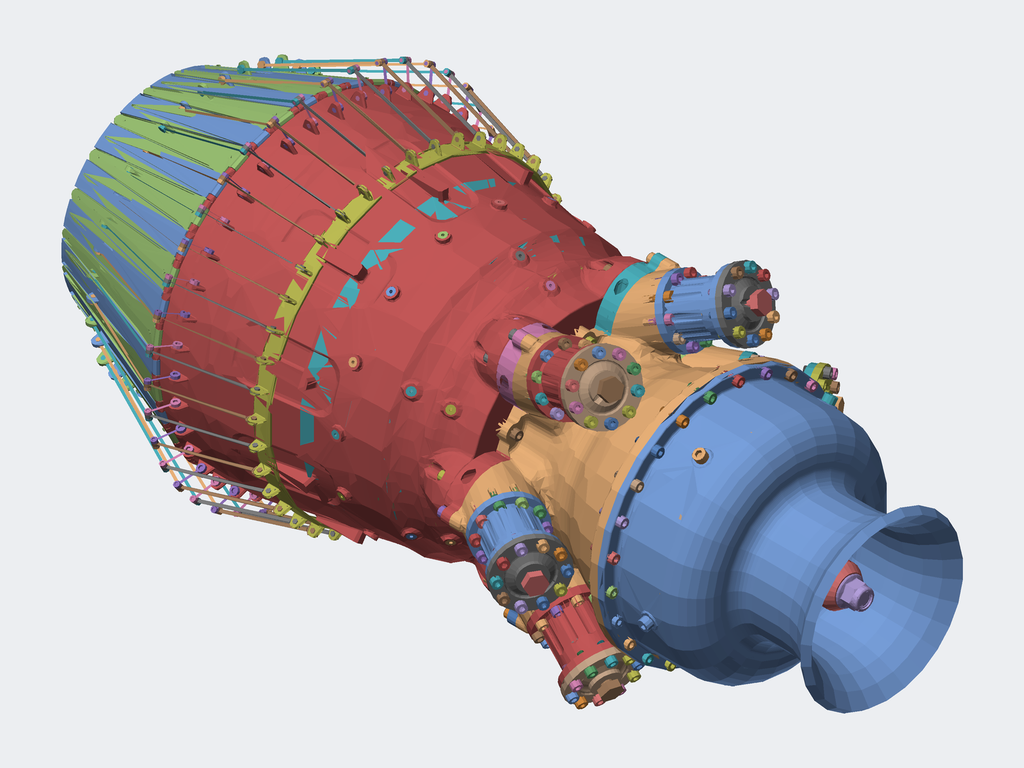Assembly | STEP file | 365 different items | 517 placed
Parts list (item | name | quantity | parent item | size | volume), first 214 of 365 items:
1 | Completa.sldasm-Part-1_Valor predeterminado (subassembly) | x1 | in Completa | 29.178 x 23 x 23 mm | 4698 mm3
2 | Completa.sldasm-Part-2_Valor predeterminado (subassembly) | x1 | in Completa | 40.919 x 104.793 x 101.882 mm | 59946 mm3
3 | Completa.sldasm-Part-3_Valor predeterminado (subassembly) | x1 | in Completa | 94.392 x 66 x 66 mm | 40484 mm3
4 | Completa.sldasm-Part-4_Valor predeterminado (subassembly) | x1 | in Completa | 21.228 x 16 x 16 mm | 1867 mm3
5 | Completa.sldasm-Part-5_Valor predeterminado (subassembly) | x1 | in Completa | 64.439 x 12 x 12 mm | 6023 mm3
6 | Completa.sldasm-Part-6_Valor predeterminado (subassembly) | x1 | in Completa | 23.351 x 16 x 16 mm | 2054 mm3
7 | Completa.sldasm-Part-7_Valor predeterminado (subassembly) | x1 | in Completa | 21.228 x 16 x 16 mm | 1867 mm3
8 | Completa.sldasm-Part-8_Valor predeterminado (subassembly) | x1 | in Completa | 64.439 x 12 x 12 mm | 6023 mm3
9 | Completa.sldasm-Part-9_Valor predeterminado (subassembly) | x1 | in Completa | 23.351 x 16 x 16 mm | 2054 mm3
10 | Completa.sldasm-Part-10_Valor predeterminado (subassembly) | x1 | in Completa | 21.228 x 16 x 16 mm | 1867 mm3
11 | Completa.sldasm-Part-11_Valor predeterminado (subassembly) | x1 | in Completa | 64.439 x 12 x 12 mm | 6023 mm3
12 | Completa.sldasm-Part-12_Valor predeterminado (subassembly) | x1 | in Completa | 23.351 x 16 x 16 mm | 2054 mm3
13 | Completa.sldasm-Part-13_Valor predeterminado (subassembly) | x1 | in Completa | 21.228 x 16 x 16 mm | 1867 mm3
14 | Completa.sldasm-Part-14_Valor predeterminado (subassembly) | x1 | in Completa | 64.439 x 12 x 12 mm | 6023 mm3
15 | Completa.sldasm-Part-15_Valor predeterminado (subassembly) | x1 | in Completa | 23.351 x 16 x 16 mm | 2054 mm3
16 | Completa.sldasm-Part-16_Valor predeterminado (subassembly) | x1 | in Completa | 23.351 x 16 x 16 mm | 2054 mm3
17 | Completa.sldasm-Part-17_Valor predeterminado (subassembly) | x1 | in Completa | 21.228 x 16 x 16 mm | 1867 mm3
18 | Completa.sldasm-Part-18_Valor predeterminado (subassembly) | x1 | in Completa | 64.439 x 12 x 12 mm | 6023 mm3
19 | Completa.sldasm-Part-19_Valor predeterminado (subassembly) | x1 | in Completa | 15.548 x 234.027 x 234.027 mm | 234749 mm3
20 | Completa.sldasm-Part-20_Valor predeterminado (subassembly) | x1 | in Completa | 7.542 x 74.256 x 74.256 mm | 20001 mm3
21 | Completa.sldasm-Part-21_Valor predeterminado (subassembly) | x1 | in Completa | 10 x 104.793 x 101.882 mm | 47802 mm3
22 | Completa.sldasm-Part-22_Valor predeterminado (subassembly) | x1 | in Completa | 260.435 x 179.116 x 179.116 mm | 192197 mm3
23 | Socket Countersunk Head Screw_ISO(ISO 10642 - M6 x 25 --- 25S)_Valor predeterminado | x1 | in Completa | 11.34 x 25.708 x 19.731 mm | 759.97 mm3
24 | Socket Countersunk Head Screw_ISO(ISO 10642 - M6 x 25 --- 25S)-1_Valor predeterminado | x1 | in Completa | 11.34 x 25.708 x 19.731 mm | 759.97 mm3
25 | Socket Countersunk Head Screw_ISO(ISO 10642 - M6 x 25 --- 25S)-2_Valor predeterminado | x1 | in Completa | 11.34 x 11.34 x 25 mm | 759.97 mm3
26 | Completa.sldasm-Part-23_Valor predeterminado (subassembly) | x1 | in Completa | 54.453 x 255.658 x 255.658 mm | 510804 mm3
27 | Completa.sldasm-Part-24_Valor predeterminado (subassembly) | x1 | in Completa | 132.616 x 276.232 x 245.091 mm | 834308 mm3
28 | Completa.sldasm-Part-25_Valor predeterminado (subassembly) | x1 | in Completa | 164.604 x 227.494 x 227.494 mm | 716979 mm3
29 | Completa.sldasm-Part-26_Valor predeterminado (subassembly) | x1 | in Completa | 13.228 x 193 x 193 mm | 129234 mm3
30 | Completa.sldasm-Part-27_Valor predeterminado (subassembly) | x1 | in Completa | 14 x 212.474 x 212.474 mm | 171916 mm3
31 | Torque nut 04-2_ISO(ISO 7043-M12-N)_Valor predeterminado | x1 | in Completa | 16.1 x 26 x 26 mm | 3173 mm3
32 | Socket Head Cap Screw_ISO(ISO 4762 M6 x 25 --- 25S)_Valor predeterminado | x1 | in Completa | 10 x 31.522 x 18.292 mm | 1014 mm3
33 | Socket Countersunk Head Screw_ISO(ISO 10642 - M6 x 25 --- 25S)-3_Valor predeterminado | x1 | in Completa | 25 x 11.34 x 11.34 mm | 759.97 mm3
34 | Socket Head Cap Screw_ISO(ISO 4762 M5 x 20 --- 20S)_Valor predeterminado | x1 | in Completa | 25 x 8.5 x 8.5 mm | 588.412 mm3
35 | Socket Head Cap Screw_ISO(ISO 4762 M5 x 20 --- 20S)-1_Valor predeterminado | x1 | in Completa | 25 x 8.5 x 8.5 mm | 588.412 mm3
36 | Socket Head Cap Screw_ISO(ISO 4762 M5 x 20 --- 20S)-2_Valor predeterminado | x1 | in Completa | 25 x 8.5 x 8.5 mm | 588.412 mm3
37 | Socket Head Cap Screw_ISO(ISO 4762 M5 x 20 --- 20S)-3_Valor predeterminado | x1 | in Completa | 25 x 8.5 x 8.5 mm | 588.412 mm3
38 | Socket Head Cap Screw_ISO(ISO 4762 M5 x 20 --- 20S)-4_Valor predeterminado | x1 | in Completa | 25 x 8.5 x 8.5 mm | 588.412 mm3
39 | Socket Head Cap Screw_ISO(ISO 4762 M5 x 20 --- 20S)-5_Valor predeterminado | x1 | in Completa | 25 x 8.5 x 8.5 mm | 588.412 mm3
40 | Socket Head Cap Screw_ISO(ISO 4762 M5 x 20 --- 20S)-6_Valor predeterminado | x1 | in Completa | 25 x 8.5 x 8.5 mm | 588.412 mm3
41 | Socket Head Cap Screw_ISO(ISO 4762 M5 x 20 --- 20S)-7_Valor predeterminado | x1 | in Completa | 25 x 8.5 x 8.5 mm | 588.412 mm3
42 | Previa 01.sldasm-Part-10_Valor predeterminado (subassembly) | x1 | in Completa | 66 x 12 x 12 mm | 6169 mm3
43 | Previa 01.sldasm-Part-16_Valor predeterminado (subassembly) | x1 | in Completa | 21.5 x 177.565 x 177.455 mm | 157095 mm3
44 | Previa 01.sldasm-Part-15_Valor predeterminado (subassembly) | x1 | in Completa | 24.229 x 188.642 x 188.976 mm | 257389 mm3
45 | Previa 01.sldasm-Part-14_Valor predeterminado (subassembly) | x1 | in Completa | 19 x 165.343 x 165.042 mm | 149848 mm3
46 | Previa 01.sldasm-Part-13_Valor predeterminado (subassembly) | x1 | in Completa | 8 x 36.3 x 36.3 mm | 5808 mm3
47 | Previa 01.sldasm-Part-11_Valor predeterminado (subassembly) | x1 | in Completa | 7 x 37.038 x 37.038 mm | 5630 mm3
48 | 003.sldasm-Part-1_Valor predeterminado (subassembly) | x1 | in Completa | 26.301 x 191 x 190.919 mm | 221330 mm3
49 | Previa 01.sldasm-Part-5_Valor predeterminado (subassembly) | x1 | in Completa | 26 x 108 x 108 mm | 90690 mm3
50 | Previa 01.sldasm-Part-4_Valor predeterminado (subassembly) | x1 | in Completa | 26.228 x 190 x 189.8 mm | 157872 mm3
51 | 003.sldasm-Part-2_Valor predeterminado (subassembly) | x1 | in Completa | 11 x 91.038 x 91.038 mm | 45789 mm3
52 | Previa 01.sldasm-Part-1_Valor predeterminado (subassembly) | x1 | in Completa | - | 182355 mm3
53 | Socket Head Cap Screw_ISO(ISO 4762 M5 x 20 --- 20S)-8_Valor predeterminado | x1 | in Completa | 19.995 x 15.067 x 8.5 mm | 493.761 mm3
54 | Socket Head Cap Screw_ISO(ISO 4762 M5 x 20 --- 20S)-9_Valor predeterminado | x1 | in Completa | 19.995 x 15.067 x 8.5 mm | 493.761 mm3
55 | Socket Head Cap Screw_ISO(ISO 4762 M5 x 20 --- 20S)-10_Valor predeterminado | x1 | in Completa | 19.995 x 15.067 x 8.5 mm | 493.761 mm3
56 | Socket Head Cap Screw_ISO(ISO 4762 M5 x 20 --- 20S)-11_Valor predeterminado | x1 | in Completa | 19.995 x 15.067 x 8.5 mm | 493.761 mm3
57 | Socket Head Cap Screw_ISO(ISO 4762 M5 x 20 --- 20S)-12_Valor predeterminado | x1 | in Completa | 19.995 x 15.067 x 8.5 mm | 493.761 mm3
58 | Socket Head Cap Screw_ISO(ISO 4762 M5 x 20 --- 20S)-13_Valor predeterminado | x1 | in Completa | 19.995 x 15.067 x 8.5 mm | 493.761 mm3
59 | Socket Head Cap Screw_ISO(ISO 4762 M5 x 20 --- 20S)-14_Valor predeterminado | x1 | in Completa | 19.995 x 15.067 x 8.5 mm | 493.761 mm3
60 | Socket Head Cap Screw_ISO(ISO 4762 M5 x 20 --- 20S)-15_Valor predeterminado | x1 | in Completa | 19.995 x 15.067 x 8.5 mm | 493.761 mm3
61 | Socket Head Cap Screw_ISO(ISO 4762 M5 x 20 --- 20S)-16_Valor predeterminado | x1 | in Completa | 19.995 x 15.067 x 8.5 mm | 493.761 mm3
62 | Socket Head Cap Screw_ISO(ISO 4762 M5 x 20 --- 20S)-17_Valor predeterminado | x1 | in Completa | 19.995 x 15.067 x 8.5 mm | 493.761 mm3
63 | Socket Head Cap Screw_ISO(ISO 4762 M5 x 20 --- 20S)-18_Valor predeterminado | x1 | in Completa | 24.833 x 17.717 x 8.5 mm | 588.412 mm3
64 | Socket Head Cap Screw_ISO(ISO 4762 M5 x 20 --- 20S)-19_Valor predeterminado | x1 | in Completa | 24.833 x 17.717 x 8.5 mm | 588.412 mm3
65 | Socket Head Cap Screw_ISO(ISO 4762 M5 x 20 --- 20S)-20_Valor predeterminado | x1 | in Completa | 24.833 x 17.717 x 8.5 mm | 588.412 mm3
66 | Socket Head Cap Screw_ISO(ISO 4762 M5 x 20 --- 20S)-21_Valor predeterminado | x1 | in Completa | 24.833 x 17.717 x 8.5 mm | 588.412 mm3
67 | Socket Head Cap Screw_ISO(ISO 4762 M5 x 20 --- 20S)-22_Valor predeterminado | x1 | in Completa | 24.833 x 17.717 x 8.5 mm | 588.412 mm3
68 | Socket Head Cap Screw_ISO(ISO 4762 M5 x 20 --- 20S)-23_Valor predeterminado | x1 | in Completa | 24.833 x 17.717 x 8.5 mm | 588.412 mm3
69 | Socket Head Cap Screw_ISO(ISO 4762 M5 x 20 --- 20S)-24_Valor predeterminado | x1 | in Completa | 24.833 x 17.717 x 8.5 mm | 588.412 mm3
70 | Socket Head Cap Screw_ISO(ISO 4762 M5 x 20 --- 20S)-25_Valor predeterminado | x1 | in Completa | 24.833 x 17.717 x 8.5 mm | 588.412 mm3
71 | Socket Head Cap Screw_ISO(ISO 4762 M5 x 20 --- 20S)-26_Valor predeterminado | x1 | in Completa | 24.833 x 17.717 x 8.5 mm | 588.412 mm3
72 | Socket Head Cap Screw_ISO(ISO 4762 M5 x 20 --- 20S)-27_Valor predeterminado | x1 | in Completa | 24.833 x 17.717 x 8.5 mm | 588.412 mm3
73 | Completa.sldasm-Part-28_Valor predeterminado (subassembly) | x1 | in Completa | 33.841 x 55.116 x 60 mm | 15153 mm3
74 | Completa.sldasm-Part-29_Valor predeterminado (subassembly) | x1 | in Completa | 74.277 x 76.616 x 59 mm | 34566 mm3
75 | Completa.sldasm-Part-30_Valor predeterminado (subassembly) | x1 | in Completa | 34.045 x 26.016 x 16 mm | 3225 mm3
76 | Completa.sldasm-Part-31_Valor predeterminado (subassembly) | x1 | in Completa | 97.324 x 73.886 x 36.376 mm | 6808 mm3
77 | Socket Countersunk Head Screw_ISO(ISO 10642 - M6 x 25 --- 25S)-4_Valor predeterminado | x1 | in Completa | 25 x 11.34 x 11.34 mm | 759.97 mm3
78 | Socket Countersunk Head Screw_ISO(ISO 10642 - M6 x 25 --- 25S)-5_Valor predeterminado | x1 | in Completa | 25 x 11.34 x 11.34 mm | 759.97 mm3
79 | Previa 01.sldasm-Part-10-1_Valor predeterminado (subassembly) | x1 | in Completa | 66 x 12 x 12 mm | 6169 mm3
80 | Socket Countersunk Head Screw_ISO(ISO 10642 - M6 x 25 --- 25S)-6_Valor predeterminado | x1 | in Completa | 25 x 11.34 x 11.34 mm | 759.97 mm3
81 | Socket Countersunk Head Screw_ISO(ISO 10642 - M6 x 25 --- 25S)-7_Valor predeterminado | x1 | in Completa | 25 x 11.34 x 11.34 mm | 759.97 mm3
82 | Previa 01.sldasm-Part-10-2_Valor predeterminado (subassembly) | x1 | in Completa | 66 x 12 x 12 mm | 6169 mm3
83 | Socket Countersunk Head Screw_ISO(ISO 10642 - M6 x 25 --- 25S)-8_Valor predeterminado | x1 | in Completa | 25 x 11.34 x 11.34 mm | 759.97 mm3
84 | Socket Countersunk Head Screw_ISO(ISO 10642 - M6 x 25 --- 25S)-9_Valor predeterminado | x1 | in Completa | 25 x 11.34 x 11.34 mm | 759.97 mm3
85 | Previa 01.sldasm-Part-10-3_Valor predeterminado (subassembly) | x1 | in Completa | 66 x 12 x 12 mm | 6169 mm3
86 | Socket Countersunk Head Screw_ISO(ISO 10642 - M6 x 25 --- 25S)-10_Valor predeterminado | x1 | in Completa | 25 x 11.34 x 11.34 mm | 759.97 mm3
87 | Socket Countersunk Head Screw_ISO(ISO 10642 - M6 x 25 --- 25S)-11_Valor predeterminado | x1 | in Completa | 25 x 11.34 x 11.34 mm | 759.97 mm3
88 | Previa 01.sldasm-Part-10-4_Valor predeterminado (subassembly) | x1 | in Completa | 66 x 12 x 12 mm | 6169 mm3
89 | Socket Countersunk Head Screw_ISO(ISO 10642 - M6 x 25 --- 25S)-12_Valor predeterminado | x1 | in Completa | 25 x 11.34 x 11.34 mm | 759.97 mm3
90 | Socket Head Cap Screw_ISO(ISO 4762 M6 x 25 --- 25S)-1_Valor predeterminado | x1 | in Completa | 10 x 25.255 x 28.655 mm | 1014 mm3
91 | Socket Head Cap Screw_ISO(ISO 4762 M6 x 25 --- 25S)-2_Valor predeterminado | x1 | in Completa | 10 x 23.176 x 29.939 mm | 1014 mm3
92 | Socket Head Cap Screw_ISO(ISO 4762 M6 x 25 --- 25S)-3_Valor predeterminado | x1 | in Completa | 10 x 31.803 x 15.54 mm | 1014 mm3
93 | Socket Head Cap Screw_ISO(ISO 4762 M6 x 25 --- 25S)-4_Valor predeterminado | x1 | in Completa | 10 x 10.285 x 31.332 mm | 1014 mm3
94 | Socket Head Cap Screw_ISO(ISO 4762 M5 x 20 --- 20S)-28_Valor predeterminado | x1 | in Completa | 24.833 x 12.447 x 16.353 mm | 588.412 mm3
95 | Socket Head Cap Screw_ISO(ISO 4762 M5 x 20 --- 20S)-29_Valor predeterminado | x1 | in Completa | 19.995 x 11.122 x 14.058 mm | 493.761 mm3
96 | Socket Head Cap Screw_ISO(ISO 4762 M5 x 20 --- 20S)-30_Valor predeterminado | x1 | in Completa | 24.833 x 12.447 x 16.353 mm | 588.412 mm3
97 | Socket Head Cap Screw_ISO(ISO 4762 M5 x 20 --- 20S)-31_Valor predeterminado | x1 | in Completa | 19.995 x 11.122 x 14.058 mm | 493.761 mm3
98 | Socket Head Cap Screw_ISO(ISO 4762 M5 x 20 --- 20S)-32_Valor predeterminado | x1 | in Completa | 19.995 x 11.122 x 14.058 mm | 493.761 mm3
99 | Socket Head Cap Screw_ISO(ISO 4762 M5 x 20 --- 20S)-33_Valor predeterminado | x1 | in Completa | 24.833 x 12.447 x 16.353 mm | 588.412 mm3
100 | Socket Head Cap Screw_ISO(ISO 4762 M5 x 20 --- 20S)-34_Valor predeterminado | x1 | in Completa | 19.995 x 11.122 x 14.058 mm | 493.761 mm3
101 | Socket Head Cap Screw_ISO(ISO 4762 M5 x 20 --- 20S)-35_Valor predeterminado | x1 | in Completa | 24.833 x 12.447 x 16.353 mm | 588.412 mm3
102 | Socket Head Cap Screw_ISO(ISO 4762 M5 x 20 --- 20S)-36_Valor predeterminado | x1 | in Completa | 19.995 x 11.122 x 14.058 mm | 493.761 mm3
103 | Socket Head Cap Screw_ISO(ISO 4762 M5 x 20 --- 20S)-37_Valor predeterminado | x1 | in Completa | 24.833 x 12.447 x 16.353 mm | 588.412 mm3
104 | Completa.sldasm-Part-32_Valor predeterminado (subassembly) | x1 | in Completa | 33.841 x 59.529 x 56.74 mm | 15153 mm3
105 | Socket Head Cap Screw_ISO(ISO 4762 M5 x 20 --- 20S)-38_Valor predeterminado | x1 | in Completa | 19.995 x 11.122 x 14.058 mm | 493.761 mm3
106 | Socket Head Cap Screw_ISO(ISO 4762 M5 x 20 --- 20S)-39_Valor predeterminado | x1 | in Completa | 19.995 x 11.122 x 14.058 mm | 493.761 mm3
107 | Socket Head Cap Screw_ISO(ISO 4762 M5 x 20 --- 20S)-40_Valor predeterminado | x1 | in Completa | 19.995 x 11.122 x 14.058 mm | 493.761 mm3
108 | Completa.sldasm-Part-33_Valor predeterminado (subassembly) | x1 | in Completa | 74.277 x 69.48 x 75.135 mm | 34566 mm3
109 | Socket Head Cap Screw_ISO(ISO 4762 M5 x 20 --- 20S)-41_Valor predeterminado | x1 | in Completa | 24.833 x 12.447 x 16.353 mm | 588.412 mm3
110 | Completa.sldasm-Part-34_Valor predeterminado (subassembly) | x1 | in Completa | 34.045 x 21.356 x 23.621 mm | 3225 mm3
111 | Socket Head Cap Screw_ISO(ISO 4762 M5 x 20 --- 20S)-42_Valor predeterminado | x1 | in Completa | 19.995 x 11.122 x 14.058 mm | 493.761 mm3
112 | Completa.sldasm-Part-35_Valor predeterminado (subassembly) | x1 | in Completa | 97.324 x 59.709 x 73.971 mm | 6808 mm3
113 | Socket Head Cap Screw_ISO(ISO 4762 M5 x 20 --- 20S)-43_Valor predeterminado | x1 | in Completa | 19.995 x 11.122 x 14.058 mm | 493.761 mm3
114 | Socket Head Cap Screw_ISO(ISO 4762 M5 x 20 --- 20S)-44_Valor predeterminado | x1 | in Completa | 24.833 x 12.447 x 16.353 mm | 588.412 mm3
115 | Socket Head Cap Screw_ISO(ISO 4762 M5 x 20 --- 20S)-45_Valor predeterminado | x1 | in Completa | 24.833 x 12.447 x 16.353 mm | 588.412 mm3
116 | Socket Head Cap Screw_ISO(ISO 4762 M5 x 20 --- 20S)-46_Valor predeterminado | x1 | in Completa | 24.833 x 12.447 x 16.353 mm | 588.412 mm3
117 | Socket Head Cap Screw_ISO(ISO 4762 M5 x 20 --- 20S)-47_Valor predeterminado | x1 | in Completa | 24.833 x 12.447 x 16.353 mm | 588.412 mm3
118 | Socket Head Cap Screw_ISO(ISO 4762 M5 x 20 --- 20S)-48_Valor predeterminado | x1 | in Completa | 24.833 x 12.447 x 16.353 mm | 588.412 mm3
119 | Socket Head Cap Screw_ISO(ISO 4762 M5 x 20 --- 20S)-49_Valor predeterminado | x1 | in Completa | 19.995 x 11.122 x 14.058 mm | 493.761 mm3
120 | Socket Head Cap Screw_ISO(ISO 4762 M5 x 20 --- 20S)-50_Valor predeterminado | x1 | in Completa | 24.833 x 12.447 x 16.353 mm | 588.412 mm3
121 | Socket Head Cap Screw_ISO(ISO 4762 M5 x 20 --- 20S)-51_Valor predeterminado | x1 | in Completa | 19.995 x 11.122 x 14.058 mm | 493.761 mm3
122 | Socket Head Cap Screw_ISO(ISO 4762 M5 x 20 --- 20S)-52_Valor predeterminado | x1 | in Completa | 19.995 x 11.122 x 14.058 mm | 493.761 mm3
123 | Socket Head Cap Screw_ISO(ISO 4762 M5 x 20 --- 20S)-53_Valor predeterminado | x1 | in Completa | 24.833 x 12.447 x 16.353 mm | 588.412 mm3
124 | Socket Head Cap Screw_ISO(ISO 4762 M5 x 20 --- 20S)-54_Valor predeterminado | x1 | in Completa | 19.995 x 11.122 x 14.058 mm | 493.761 mm3
125 | Socket Head Cap Screw_ISO(ISO 4762 M5 x 20 --- 20S)-55_Valor predeterminado | x1 | in Completa | 24.833 x 12.447 x 16.353 mm | 588.412 mm3
126 | Socket Head Cap Screw_ISO(ISO 4762 M5 x 20 --- 20S)-56_Valor predeterminado | x1 | in Completa | 19.995 x 11.122 x 14.058 mm | 493.761 mm3
127 | Socket Head Cap Screw_ISO(ISO 4762 M5 x 20 --- 20S)-57_Valor predeterminado | x1 | in Completa | 24.833 x 12.447 x 16.353 mm | 588.412 mm3
128 | Completa.sldasm-Part-36_Valor predeterminado (subassembly) | x1 | in Completa | 33.841 x 59.529 x 56.74 mm | 15153 mm3
129 | Socket Head Cap Screw_ISO(ISO 4762 M5 x 20 --- 20S)-58_Valor predeterminado | x1 | in Completa | 19.995 x 11.122 x 14.058 mm | 493.761 mm3
130 | Socket Head Cap Screw_ISO(ISO 4762 M5 x 20 --- 20S)-59_Valor predeterminado | x1 | in Completa | 19.995 x 11.122 x 14.058 mm | 493.761 mm3
131 | Socket Head Cap Screw_ISO(ISO 4762 M5 x 20 --- 20S)-60_Valor predeterminado | x1 | in Completa | 19.995 x 11.122 x 14.058 mm | 493.761 mm3
132 | Completa.sldasm-Part-37_Valor predeterminado (subassembly) | x1 | in Completa | 74.277 x 69.48 x 75.135 mm | 34566 mm3
133 | Socket Head Cap Screw_ISO(ISO 4762 M5 x 20 --- 20S)-61_Valor predeterminado | x1 | in Completa | 24.833 x 12.447 x 16.353 mm | 588.412 mm3
134 | Completa.sldasm-Part-38_Valor predeterminado (subassembly) | x1 | in Completa | 34.045 x 21.356 x 23.621 mm | 3225 mm3
135 | Socket Head Cap Screw_ISO(ISO 4762 M5 x 20 --- 20S)-62_Valor predeterminado | x1 | in Completa | 19.995 x 11.122 x 14.058 mm | 493.761 mm3
136 | Completa.sldasm-Part-39_Valor predeterminado (subassembly) | x1 | in Completa | 97.324 x 59.709 x 73.971 mm | 6808 mm3
137 | Socket Head Cap Screw_ISO(ISO 4762 M5 x 20 --- 20S)-63_Valor predeterminado | x1 | in Completa | 19.995 x 11.122 x 14.058 mm | 493.761 mm3
138 | Socket Head Cap Screw_ISO(ISO 4762 M5 x 20 --- 20S)-64_Valor predeterminado | x1 | in Completa | 24.833 x 12.447 x 16.353 mm | 588.412 mm3
139 | Socket Head Cap Screw_ISO(ISO 4762 M5 x 20 --- 20S)-65_Valor predeterminado | x1 | in Completa | 24.833 x 12.447 x 16.353 mm | 588.412 mm3
140 | Socket Head Cap Screw_ISO(ISO 4762 M5 x 20 --- 20S)-66_Valor predeterminado | x1 | in Completa | 24.833 x 12.447 x 16.353 mm | 588.412 mm3
141 | Socket Head Cap Screw_ISO(ISO 4762 M5 x 20 --- 20S)-67_Valor predeterminado | x1 | in Completa | 24.833 x 12.447 x 16.353 mm | 588.412 mm3
142 | Socket Head Cap Screw_ISO(ISO 4762 M5 x 20 --- 20S)-68_Valor predeterminado | x1 | in Completa | 24.833 x 17.717 x 8.5 mm | 588.412 mm3
143 | Socket Head Cap Screw_ISO(ISO 4762 M5 x 20 --- 20S)-69_Valor predeterminado | x1 | in Completa | 19.995 x 15.067 x 8.5 mm | 493.761 mm3
144 | Socket Head Cap Screw_ISO(ISO 4762 M5 x 20 --- 20S)-70_Valor predeterminado | x1 | in Completa | 24.833 x 17.717 x 8.5 mm | 588.412 mm3
145 | Socket Head Cap Screw_ISO(ISO 4762 M5 x 20 --- 20S)-71_Valor predeterminado | x1 | in Completa | 19.995 x 15.067 x 8.5 mm | 493.761 mm3
146 | Socket Head Cap Screw_ISO(ISO 4762 M5 x 20 --- 20S)-72_Valor predeterminado | x1 | in Completa | 19.995 x 15.067 x 8.5 mm | 493.761 mm3
147 | Socket Head Cap Screw_ISO(ISO 4762 M5 x 20 --- 20S)-73_Valor predeterminado | x1 | in Completa | 24.833 x 17.717 x 8.5 mm | 588.412 mm3
148 | Socket Head Cap Screw_ISO(ISO 4762 M5 x 20 --- 20S)-74_Valor predeterminado | x1 | in Completa | 19.995 x 15.067 x 8.5 mm | 493.761 mm3
149 | Socket Head Cap Screw_ISO(ISO 4762 M5 x 20 --- 20S)-75_Valor predeterminado | x1 | in Completa | 24.833 x 17.717 x 8.5 mm | 588.412 mm3
150 | Socket Head Cap Screw_ISO(ISO 4762 M5 x 20 --- 20S)-76_Valor predeterminado | x1 | in Completa | 19.995 x 15.067 x 8.5 mm | 493.761 mm3
151 | Socket Head Cap Screw_ISO(ISO 4762 M5 x 20 --- 20S)-77_Valor predeterminado | x1 | in Completa | 24.833 x 17.717 x 8.5 mm | 588.412 mm3
152 | Completa.sldasm-Part-40_Valor predeterminado (subassembly) | x1 | in Completa | 33.841 x 55.116 x 60 mm | 15153 mm3
153 | Socket Head Cap Screw_ISO(ISO 4762 M5 x 20 --- 20S)-78_Valor predeterminado | x1 | in Completa | 19.995 x 15.067 x 8.5 mm | 493.761 mm3
154 | Socket Head Cap Screw_ISO(ISO 4762 M5 x 20 --- 20S)-79_Valor predeterminado | x1 | in Completa | 19.995 x 15.067 x 8.5 mm | 493.761 mm3
155 | Socket Head Cap Screw_ISO(ISO 4762 M5 x 20 --- 20S)-80_Valor predeterminado | x1 | in Completa | 19.995 x 15.067 x 8.5 mm | 493.761 mm3
156 | Completa.sldasm-Part-41_Valor predeterminado (subassembly) | x1 | in Completa | 74.277 x 76.616 x 59 mm | 34566 mm3
157 | Socket Head Cap Screw_ISO(ISO 4762 M5 x 20 --- 20S)-81_Valor predeterminado | x1 | in Completa | 24.833 x 17.717 x 8.5 mm | 588.412 mm3
158 | Completa.sldasm-Part-42_Valor predeterminado (subassembly) | x1 | in Completa | 34.045 x 26.016 x 16 mm | 3225 mm3
159 | Socket Head Cap Screw_ISO(ISO 4762 M5 x 20 --- 20S)-82_Valor predeterminado | x1 | in Completa | 19.995 x 15.067 x 8.5 mm | 493.761 mm3
160 | Completa.sldasm-Part-43_Valor predeterminado (subassembly) | x1 | in Completa | 97.324 x 73.886 x 36.376 mm | 6808 mm3
161 | Socket Head Cap Screw_ISO(ISO 4762 M5 x 20 --- 20S)-83_Valor predeterminado | x1 | in Completa | 19.995 x 15.067 x 8.5 mm | 493.761 mm3
162 | Socket Head Cap Screw_ISO(ISO 4762 M5 x 20 --- 20S)-84_Valor predeterminado | x1 | in Completa | 24.833 x 17.717 x 8.5 mm | 588.412 mm3
163 | Socket Head Cap Screw_ISO(ISO 4762 M5 x 20 --- 20S)-85_Valor predeterminado | x1 | in Completa | 24.833 x 17.717 x 8.5 mm | 588.412 mm3
164 | Socket Head Cap Screw_ISO(ISO 4762 M5 x 20 --- 20S)-86_Valor predeterminado | x1 | in Completa | 24.833 x 17.717 x 8.5 mm | 588.412 mm3
165 | Socket Head Cap Screw_ISO(ISO 4762 M5 x 20 --- 20S)-87_Valor predeterminado | x1 | in Completa | 24.833 x 17.717 x 8.5 mm | 588.412 mm3
166 | Socket Head Cap Screw_ISO(ISO 4762 M5 x 20 --- 20S)-88_Valor predeterminado | x1 | in Completa | 24.833 x 12.447 x 16.353 mm | 588.412 mm3
167 | Socket Head Cap Screw_ISO(ISO 4762 M5 x 20 --- 20S)-89_Valor predeterminado | x1 | in Completa | 19.995 x 11.122 x 14.058 mm | 493.761 mm3
168 | Socket Head Cap Screw_ISO(ISO 4762 M5 x 20 --- 20S)-90_Valor predeterminado | x1 | in Completa | 24.833 x 12.447 x 16.353 mm | 588.412 mm3
169 | Socket Head Cap Screw_ISO(ISO 4762 M5 x 20 --- 20S)-91_Valor predeterminado | x1 | in Completa | 19.995 x 11.122 x 14.058 mm | 493.761 mm3
170 | Socket Head Cap Screw_ISO(ISO 4762 M5 x 20 --- 20S)-92_Valor predeterminado | x1 | in Completa | 19.995 x 11.122 x 14.058 mm | 493.761 mm3
171 | Socket Head Cap Screw_ISO(ISO 4762 M5 x 20 --- 20S)-93_Valor predeterminado | x1 | in Completa | 24.833 x 12.447 x 16.353 mm | 588.412 mm3
172 | Socket Head Cap Screw_ISO(ISO 4762 M5 x 20 --- 20S)-94_Valor predeterminado | x1 | in Completa | 19.995 x 11.122 x 14.058 mm | 493.761 mm3
173 | Socket Head Cap Screw_ISO(ISO 4762 M5 x 20 --- 20S)-95_Valor predeterminado | x1 | in Completa | 24.833 x 12.447 x 16.353 mm | 588.412 mm3
174 | Socket Head Cap Screw_ISO(ISO 4762 M5 x 20 --- 20S)-96_Valor predeterminado | x1 | in Completa | 19.995 x 11.122 x 14.058 mm | 493.761 mm3
175 | Socket Head Cap Screw_ISO(ISO 4762 M5 x 20 --- 20S)-97_Valor predeterminado | x1 | in Completa | 24.833 x 12.447 x 16.353 mm | 588.412 mm3
176 | Completa.sldasm-Part-44_Valor predeterminado (subassembly) | x1 | in Completa | 33.841 x 59.529 x 56.74 mm | 15153 mm3
177 | Socket Head Cap Screw_ISO(ISO 4762 M5 x 20 --- 20S)-98_Valor predeterminado | x1 | in Completa | 19.995 x 11.122 x 14.058 mm | 493.761 mm3
178 | Socket Head Cap Screw_ISO(ISO 4762 M5 x 20 --- 20S)-99_Valor predeterminado | x1 | in Completa | 19.995 x 11.122 x 14.058 mm | 493.761 mm3
179 | Socket Head Cap Screw_ISO(ISO 4762 M5 x 20 --- 20S)-100_Valor predeterminado | x1 | in Completa | 19.995 x 11.122 x 14.058 mm | 493.761 mm3
180 | Completa.sldasm-Part-45_Valor predeterminado (subassembly) | x1 | in Completa | 74.277 x 69.48 x 75.135 mm | 34566 mm3
181 | Socket Head Cap Screw_ISO(ISO 4762 M5 x 20 --- 20S)-101_Valor predeterminado | x1 | in Completa | 24.833 x 12.447 x 16.353 mm | 588.412 mm3
182 | Completa.sldasm-Part-46_Valor predeterminado (subassembly) | x1 | in Completa | 34.045 x 21.356 x 23.621 mm | 3225 mm3
183 | Socket Head Cap Screw_ISO(ISO 4762 M5 x 20 --- 20S)-102_Valor predeterminado | x1 | in Completa | 19.995 x 11.122 x 14.058 mm | 493.761 mm3
184 | Completa.sldasm-Part-47_Valor predeterminado (subassembly) | x1 | in Completa | 97.324 x 59.709 x 73.971 mm | 6808 mm3
185 | Socket Head Cap Screw_ISO(ISO 4762 M5 x 20 --- 20S)-103_Valor predeterminado | x1 | in Completa | 19.995 x 11.122 x 14.058 mm | 493.761 mm3
186 | Socket Head Cap Screw_ISO(ISO 4762 M5 x 20 --- 20S)-104_Valor predeterminado | x1 | in Completa | 24.833 x 12.447 x 16.353 mm | 588.412 mm3
187 | Socket Head Cap Screw_ISO(ISO 4762 M5 x 20 --- 20S)-105_Valor predeterminado | x1 | in Completa | 24.833 x 12.447 x 16.353 mm | 588.412 mm3
188 | Socket Head Cap Screw_ISO(ISO 4762 M5 x 20 --- 20S)-106_Valor predeterminado | x1 | in Completa | 24.833 x 12.447 x 16.353 mm | 588.412 mm3
189 | Socket Head Cap Screw_ISO(ISO 4762 M5 x 20 --- 20S)-107_Valor predeterminado | x1 | in Completa | 24.833 x 12.447 x 16.353 mm | 588.412 mm3
190 | Socket Head Cap Screw_ISO(ISO 4762 M5 x 20 --- 20S)-108_Valor predeterminado | x1 | in Completa | 24.833 x 12.447 x 16.353 mm | 588.412 mm3
191 | Socket Head Cap Screw_ISO(ISO 4762 M5 x 20 --- 20S)-109_Valor predeterminado | x1 | in Completa | 19.995 x 11.122 x 14.058 mm | 493.761 mm3
192 | Socket Head Cap Screw_ISO(ISO 4762 M5 x 20 --- 20S)-110_Valor predeterminado | x1 | in Completa | 24.833 x 12.447 x 16.353 mm | 588.412 mm3
193 | Socket Head Cap Screw_ISO(ISO 4762 M5 x 20 --- 20S)-111_Valor predeterminado | x1 | in Completa | 19.995 x 11.122 x 14.058 mm | 493.761 mm3
194 | Socket Head Cap Screw_ISO(ISO 4762 M5 x 20 --- 20S)-112_Valor predeterminado | x1 | in Completa | 19.995 x 11.122 x 14.058 mm | 493.761 mm3
195 | Socket Head Cap Screw_ISO(ISO 4762 M5 x 20 --- 20S)-113_Valor predeterminado | x1 | in Completa | 24.833 x 12.447 x 16.353 mm | 588.412 mm3
196 | Socket Head Cap Screw_ISO(ISO 4762 M5 x 20 --- 20S)-114_Valor predeterminado | x1 | in Completa | 19.995 x 11.122 x 14.058 mm | 493.761 mm3
197 | Socket Head Cap Screw_ISO(ISO 4762 M5 x 20 --- 20S)-115_Valor predeterminado | x1 | in Completa | 24.833 x 12.447 x 16.353 mm | 588.412 mm3
198 | Socket Head Cap Screw_ISO(ISO 4762 M5 x 20 --- 20S)-116_Valor predeterminado | x1 | in Completa | 19.995 x 11.122 x 14.058 mm | 493.761 mm3
199 | Socket Head Cap Screw_ISO(ISO 4762 M5 x 20 --- 20S)-117_Valor predeterminado | x1 | in Completa | 24.833 x 12.447 x 16.353 mm | 588.412 mm3
200 | Completa.sldasm-Part-48_Valor predeterminado (subassembly) | x1 | in Completa | 33.841 x 59.529 x 56.74 mm | 15153 mm3
201 | Socket Head Cap Screw_ISO(ISO 4762 M5 x 20 --- 20S)-118_Valor predeterminado | x1 | in Completa | 19.995 x 11.122 x 14.058 mm | 493.761 mm3
202 | Socket Head Cap Screw_ISO(ISO 4762 M5 x 20 --- 20S)-119_Valor predeterminado | x1 | in Completa | 19.995 x 11.122 x 14.058 mm | 493.761 mm3
203 | Socket Head Cap Screw_ISO(ISO 4762 M5 x 20 --- 20S)-120_Valor predeterminado | x1 | in Completa | 19.995 x 11.122 x 14.058 mm | 493.761 mm3
204 | Completa.sldasm-Part-49_Valor predeterminado (subassembly) | x1 | in Completa | 74.277 x 69.48 x 75.135 mm | 34566 mm3
205 | Socket Head Cap Screw_ISO(ISO 4762 M5 x 20 --- 20S)-121_Valor predeterminado | x1 | in Completa | 24.833 x 12.447 x 16.353 mm | 588.412 mm3
206 | Completa.sldasm-Part-50_Valor predeterminado (subassembly) | x1 | in Completa | 34.045 x 21.356 x 23.621 mm | 3225 mm3
207 | Socket Head Cap Screw_ISO(ISO 4762 M5 x 20 --- 20S)-122_Valor predeterminado | x1 | in Completa | 19.995 x 11.122 x 14.058 mm | 493.761 mm3
208 | Completa.sldasm-Part-51_Valor predeterminado (subassembly) | x1 | in Completa | 97.324 x 59.709 x 73.971 mm | 6808 mm3
209 | Socket Head Cap Screw_ISO(ISO 4762 M5 x 20 --- 20S)-123_Valor predeterminado | x1 | in Completa | 19.995 x 11.122 x 14.058 mm | 493.761 mm3
210 | Socket Head Cap Screw_ISO(ISO 4762 M5 x 20 --- 20S)-124_Valor predeterminado | x1 | in Completa | 24.833 x 12.447 x 16.353 mm | 588.412 mm3
211 | Socket Head Cap Screw_ISO(ISO 4762 M5 x 20 --- 20S)-125_Valor predeterminado | x1 | in Completa | 24.833 x 12.447 x 16.353 mm | 588.412 mm3
212 | Socket Head Cap Screw_ISO(ISO 4762 M5 x 20 --- 20S)-126_Valor predeterminado | x1 | in Completa | 24.833 x 12.447 x 16.353 mm | 588.412 mm3
213 | Socket Head Cap Screw_ISO(ISO 4762 M5 x 20 --- 20S)-127_Valor predeterminado | x1 | in Completa | 24.833 x 12.447 x 16.353 mm | 588.412 mm3
214 | Previa 01.sldasm-Part-6_Valor predeterminado (subassembly) | x1 | in Completa | 15 x 108.559 x 108.559 mm | 81796 mm3
Placements (level | parent | child | x y z in mm | rotation matrix by rows), first 157 of 517 lines:
1 | Completa | Completa.sldasm-Part-1_Valor predeterminado | -0.0 -0.0 -0.0 | 1 0 0 0 1 0 0 0 1
1 | Completa | Completa.sldasm-Part-2_Valor predeterminado | -0.0 -0.0 -0.0 | 1 0 0 0 1 0 0 0 1
1 | Completa | Completa.sldasm-Part-3_Valor predeterminado | -0.0 -0.0 -0.0 | 1 0 0 0 1 0 0 0 1
1 | Completa | Completa.sldasm-Part-4_Valor predeterminado | -0.0 -0.0 -0.0 | 1 0 0 0 1 0 0 0 1
1 | Completa | Completa.sldasm-Part-5_Valor predeterminado | -0.0 -0.0 -0.0 | 1 0 0 0 1 0 0 0 1
1 | Completa | Completa.sldasm-Part-6_Valor predeterminado | -0.0 -0.0 -0.0 | 1 0 0 0 1 0 0 0 1
1 | Completa | Completa.sldasm-Part-7_Valor predeterminado | -0.0 -0.0 -0.0 | 1 0 0 0 1 0 0 0 1
1 | Completa | Completa.sldasm-Part-8_Valor predeterminado | -0.0 -0.0 -0.0 | 1 0 0 0 1 0 0 0 1
1 | Completa | Completa.sldasm-Part-9_Valor predeterminado | -0.0 -0.0 -0.0 | 1 0 0 0 1 0 0 0 1
1 | Completa | Completa.sldasm-Part-10_Valor predeterminado | -0.0 -0.0 -0.0 | 1 0 0 0 1 0 0 0 1
1 | Completa | Completa.sldasm-Part-11_Valor predeterminado | -0.0 -0.0 -0.0 | 1 0 0 0 1 0 0 0 1
1 | Completa | Completa.sldasm-Part-12_Valor predeterminado | -0.0 -0.0 -0.0 | 1 0 0 0 1 0 0 0 1
1 | Completa | Completa.sldasm-Part-13_Valor predeterminado | -0.0 -0.0 -0.0 | 1 0 0 0 1 0 0 0 1
1 | Completa | Completa.sldasm-Part-14_Valor predeterminado | -0.0 -0.0 -0.0 | 1 0 0 0 1 0 0 0 1
1 | Completa | Completa.sldasm-Part-15_Valor predeterminado | -0.0 -0.0 -0.0 | 1 0 0 0 1 0 0 0 1
1 | Completa | Completa.sldasm-Part-16_Valor predeterminado | -0.0 -0.0 -0.0 | 1 0 0 0 1 0 0 0 1
1 | Completa | Completa.sldasm-Part-17_Valor predeterminado | -0.0 -0.0 -0.0 | 1 0 0 0 1 0 0 0 1
1 | Completa | Completa.sldasm-Part-18_Valor predeterminado | -0.0 -0.0 -0.0 | 1 0 0 0 1 0 0 0 1
1 | Completa | Completa.sldasm-Part-19_Valor predeterminado | -0.0 -0.0 -0.0 | 1 0 0 0 1 0 0 0 1
1 | Completa | Completa.sldasm-Part-20_Valor predeterminado | -0.0 -0.0 -0.0 | 1 0 0 0 1 0 0 0 1
1 | Completa | Completa.sldasm-Part-21_Valor predeterminado | -0.0 -0.0 -0.0 | 1 0 0 0 1 0 0 0 1
1 | Completa | Completa.sldasm-Part-22_Valor predeterminado | -0.0 -0.0 -0.0 | 1 0 0 0 1 0 0 0 1
1 | Completa | Socket Countersunk Head Screw_ISO(ISO 10642 - M6 x 25 --- 25S)_Valor predeterminado | -0.0 -0.0 -0.0 | 1 0 0 0 1 0 0 0 1
1 | Completa | Socket Countersunk Head Screw_ISO(ISO 10642 - M6 x 25 --- 25S)-1_Valor predeterminado | -0.0 -0.0 -0.0 | 1 0 0 0 1 0 0 0 1
1 | Completa | Socket Countersunk Head Screw_ISO(ISO 10642 - M6 x 25 --- 25S)-2_Valor predeterminado | -0.0 -0.0 -0.0 | 1 0 0 0 1 0 0 0 1
1 | Completa | Completa.sldasm-Part-23_Valor predeterminado | -0.0 -0.0 -0.0 | 1 0 0 0 1 0 0 0 1
1 | Completa | Completa.sldasm-Part-24_Valor predeterminado | -0.0 -0.0 -0.0 | 1 0 0 0 1 0 0 0 1
1 | Completa | Completa.sldasm-Part-25_Valor predeterminado | -0.0 -0.0 -0.0 | 1 0 0 0 1 0 0 0 1
1 | Completa | Completa.sldasm-Part-26_Valor predeterminado | -0.0 -0.0 -0.0 | 1 0 0 0 1 0 0 0 1
1 | Completa | Completa.sldasm-Part-27_Valor predeterminado | -0.0 -0.0 -0.0 | 1 0 0 0 1 0 0 0 1
1 | Completa | Torque nut 04-2_ISO(ISO 7043-M12-N)_Valor predeterminado | -0.0 -0.0 -0.0 | 1 0 0 0 1 0 0 0 1
1 | Completa | Socket Head Cap Screw_ISO(ISO 4762 M6 x 25 --- 25S)_Valor predeterminado | -0.0 -0.0 -0.0 | 1 0 0 0 1 0 0 0 1
1 | Completa | Socket Countersunk Head Screw_ISO(ISO 10642 - M6 x 25 --- 25S)-3_Valor predeterminado | -0.0 -0.0 -0.0 | 1 0 0 0 1 0 0 0 1
1 | Completa | Socket Head Cap Screw_ISO(ISO 4762 M5 x 20 --- 20S)_Valor predeterminado | -0.0 -0.0 -0.0 | 1 0 0 0 1 0 0 0 1
1 | Completa | Socket Head Cap Screw_ISO(ISO 4762 M5 x 20 --- 20S)-1_Valor predeterminado | -0.0 -0.0 -0.0 | 1 0 0 0 1 0 0 0 1
1 | Completa | Socket Head Cap Screw_ISO(ISO 4762 M5 x 20 --- 20S)-2_Valor predeterminado | -0.0 -0.0 -0.0 | 1 0 0 0 1 0 0 0 1
1 | Completa | Socket Head Cap Screw_ISO(ISO 4762 M5 x 20 --- 20S)-3_Valor predeterminado | -0.0 -0.0 -0.0 | 1 0 0 0 1 0 0 0 1
1 | Completa | Socket Head Cap Screw_ISO(ISO 4762 M5 x 20 --- 20S)-4_Valor predeterminado | -0.0 -0.0 -0.0 | 1 0 0 0 1 0 0 0 1
1 | Completa | Socket Head Cap Screw_ISO(ISO 4762 M5 x 20 --- 20S)-5_Valor predeterminado | -0.0 -0.0 -0.0 | 1 0 0 0 1 0 0 0 1
1 | Completa | Socket Head Cap Screw_ISO(ISO 4762 M5 x 20 --- 20S)-6_Valor predeterminado | -0.0 -0.0 -0.0 | 1 0 0 0 1 0 0 0 1
1 | Completa | Socket Head Cap Screw_ISO(ISO 4762 M5 x 20 --- 20S)-7_Valor predeterminado | -0.0 -0.0 -0.0 | 1 0 0 0 1 0 0 0 1
1 | Completa | Previa 01.sldasm-Part-10_Valor predeterminado | -0.0 -0.0 -0.0 | 1 0 0 0 1 0 0 0 1
1 | Completa | Previa 01.sldasm-Part-16_Valor predeterminado | -0.0 -0.0 -0.0 | 1 0 0 0 1 0 0 0 1
1 | Completa | Previa 01.sldasm-Part-15_Valor predeterminado | -0.0 -0.0 -0.0 | 1 0 0 0 1 0 0 0 1
1 | Completa | Previa 01.sldasm-Part-14_Valor predeterminado | -0.0 -0.0 -0.0 | 1 0 0 0 1 0 0 0 1
1 | Completa | Previa 01.sldasm-Part-13_Valor predeterminado | -0.0 -0.0 -0.0 | 1 0 0 0 1 0 0 0 1
1 | Completa | Previa 01.sldasm-Part-11_Valor predeterminado | -0.0 -0.0 -0.0 | 1 0 0 0 1 0 0 0 1
1 | Completa | 003.sldasm-Part-1_Valor predeterminado | -0.0 -0.0 -0.0 | 1 0 0 0 1 0 0 0 1
1 | Completa | Previa 01.sldasm-Part-5_Valor predeterminado | -0.0 -0.0 -0.0 | 1 0 0 0 1 0 0 0 1
1 | Completa | Previa 01.sldasm-Part-4_Valor predeterminado | -0.0 -0.0 -0.0 | 1 0 0 0 1 0 0 0 1
1 | Completa | 003.sldasm-Part-2_Valor predeterminado | -0.0 -0.0 -0.0 | 1 0 0 0 1 0 0 0 1
1 | Completa | Previa 01.sldasm-Part-1_Valor predeterminado | -0.0 -0.0 -0.0 | 1 0 0 0 1 0 0 0 1
1 | Completa | Socket Head Cap Screw_ISO(ISO 4762 M5 x 20 --- 20S)-8_Valor predeterminado | -0.0 -0.0 -0.0 | 1 0 0 0 1 0 0 0 1
1 | Completa | Socket Head Cap Screw_ISO(ISO 4762 M5 x 20 --- 20S)-9_Valor predeterminado | -0.0 -0.0 -0.0 | 1 0 0 0 1 0 0 0 1
1 | Completa | Socket Head Cap Screw_ISO(ISO 4762 M5 x 20 --- 20S)-10_Valor predeterminado | -0.0 -0.0 -0.0 | 1 0 0 0 1 0 0 0 1
1 | Completa | Socket Head Cap Screw_ISO(ISO 4762 M5 x 20 --- 20S)-11_Valor predeterminado | -0.0 -0.0 -0.0 | 1 0 0 0 1 0 0 0 1
1 | Completa | Socket Head Cap Screw_ISO(ISO 4762 M5 x 20 --- 20S)-12_Valor predeterminado | -0.0 -0.0 -0.0 | 1 0 0 0 1 0 0 0 1
1 | Completa | Socket Head Cap Screw_ISO(ISO 4762 M5 x 20 --- 20S)-13_Valor predeterminado | -0.0 -0.0 -0.0 | 1 0 0 0 1 0 0 0 1
1 | Completa | Socket Head Cap Screw_ISO(ISO 4762 M5 x 20 --- 20S)-14_Valor predeterminado | -0.0 -0.0 -0.0 | 1 0 0 0 1 0 0 0 1
1 | Completa | Socket Head Cap Screw_ISO(ISO 4762 M5 x 20 --- 20S)-15_Valor predeterminado | -0.0 -0.0 -0.0 | 1 0 0 0 1 0 0 0 1
1 | Completa | Socket Head Cap Screw_ISO(ISO 4762 M5 x 20 --- 20S)-16_Valor predeterminado | -0.0 -0.0 -0.0 | 1 0 0 0 1 0 0 0 1
1 | Completa | Socket Head Cap Screw_ISO(ISO 4762 M5 x 20 --- 20S)-17_Valor predeterminado | -0.0 -0.0 -0.0 | 1 0 0 0 1 0 0 0 1
1 | Completa | Socket Head Cap Screw_ISO(ISO 4762 M5 x 20 --- 20S)-18_Valor predeterminado | -0.0 -0.0 -0.0 | 1 0 0 0 1 0 0 0 1
1 | Completa | Socket Head Cap Screw_ISO(ISO 4762 M5 x 20 --- 20S)-19_Valor predeterminado | -0.0 -0.0 -0.0 | 1 0 0 0 1 0 0 0 1
1 | Completa | Socket Head Cap Screw_ISO(ISO 4762 M5 x 20 --- 20S)-20_Valor predeterminado | -0.0 -0.0 -0.0 | 1 0 0 0 1 0 0 0 1
1 | Completa | Socket Head Cap Screw_ISO(ISO 4762 M5 x 20 --- 20S)-21_Valor predeterminado | -0.0 -0.0 -0.0 | 1 0 0 0 1 0 0 0 1
1 | Completa | Socket Head Cap Screw_ISO(ISO 4762 M5 x 20 --- 20S)-22_Valor predeterminado | -0.0 -0.0 -0.0 | 1 0 0 0 1 0 0 0 1
1 | Completa | Socket Head Cap Screw_ISO(ISO 4762 M5 x 20 --- 20S)-23_Valor predeterminado | -0.0 -0.0 -0.0 | 1 0 0 0 1 0 0 0 1
1 | Completa | Socket Head Cap Screw_ISO(ISO 4762 M5 x 20 --- 20S)-24_Valor predeterminado | -0.0 -0.0 -0.0 | 1 0 0 0 1 0 0 0 1
1 | Completa | Socket Head Cap Screw_ISO(ISO 4762 M5 x 20 --- 20S)-25_Valor predeterminado | -0.0 -0.0 -0.0 | 1 0 0 0 1 0 0 0 1
1 | Completa | Socket Head Cap Screw_ISO(ISO 4762 M5 x 20 --- 20S)-26_Valor predeterminado | -0.0 -0.0 -0.0 | 1 0 0 0 1 0 0 0 1
1 | Completa | Socket Head Cap Screw_ISO(ISO 4762 M5 x 20 --- 20S)-27_Valor predeterminado | -0.0 -0.0 -0.0 | 1 0 0 0 1 0 0 0 1
1 | Completa | Completa.sldasm-Part-28_Valor predeterminado | -0.0 -0.0 -0.0 | 1 0 0 0 1 0 0 0 1
1 | Completa | Completa.sldasm-Part-29_Valor predeterminado | -0.0 -0.0 -0.0 | 1 0 0 0 1 0 0 0 1
1 | Completa | Completa.sldasm-Part-30_Valor predeterminado | -0.0 -0.0 -0.0 | 1 0 0 0 1 0 0 0 1
1 | Completa | Completa.sldasm-Part-31_Valor predeterminado | -0.0 -0.0 -0.0 | 1 0 0 0 1 0 0 0 1
1 | Completa | Socket Countersunk Head Screw_ISO(ISO 10642 - M6 x 25 --- 25S)-4_Valor predeterminado | -0.0 -0.0 -0.0 | 1 0 0 0 1 0 0 0 1
1 | Completa | Socket Countersunk Head Screw_ISO(ISO 10642 - M6 x 25 --- 25S)-5_Valor predeterminado | -0.0 -0.0 -0.0 | 1 0 0 0 1 0 0 0 1
1 | Completa | Previa 01.sldasm-Part-10-1_Valor predeterminado | -0.0 -0.0 -0.0 | 1 0 0 0 1 0 0 0 1
1 | Completa | Socket Countersunk Head Screw_ISO(ISO 10642 - M6 x 25 --- 25S)-6_Valor predeterminado | -0.0 -0.0 -0.0 | 1 0 0 0 1 0 0 0 1
1 | Completa | Socket Countersunk Head Screw_ISO(ISO 10642 - M6 x 25 --- 25S)-7_Valor predeterminado | -0.0 -0.0 -0.0 | 1 0 0 0 1 0 0 0 1
1 | Completa | Previa 01.sldasm-Part-10-2_Valor predeterminado | -0.0 -0.0 -0.0 | 1 0 0 0 1 0 0 0 1
1 | Completa | Socket Countersunk Head Screw_ISO(ISO 10642 - M6 x 25 --- 25S)-8_Valor predeterminado | -0.0 -0.0 -0.0 | 1 0 0 0 1 0 0 0 1
1 | Completa | Socket Countersunk Head Screw_ISO(ISO 10642 - M6 x 25 --- 25S)-9_Valor predeterminado | -0.0 -0.0 -0.0 | 1 0 0 0 1 0 0 0 1
1 | Completa | Previa 01.sldasm-Part-10-3_Valor predeterminado | -0.0 -0.0 -0.0 | 1 0 0 0 1 0 0 0 1
1 | Completa | Socket Countersunk Head Screw_ISO(ISO 10642 - M6 x 25 --- 25S)-10_Valor predeterminado | -0.0 -0.0 -0.0 | 1 0 0 0 1 0 0 0 1
1 | Completa | Socket Countersunk Head Screw_ISO(ISO 10642 - M6 x 25 --- 25S)-11_Valor predeterminado | -0.0 -0.0 -0.0 | 1 0 0 0 1 0 0 0 1
1 | Completa | Previa 01.sldasm-Part-10-4_Valor predeterminado | -0.0 -0.0 -0.0 | 1 0 0 0 1 0 0 0 1
1 | Completa | Socket Countersunk Head Screw_ISO(ISO 10642 - M6 x 25 --- 25S)-12_Valor predeterminado | -0.0 -0.0 -0.0 | 1 0 0 0 1 0 0 0 1
1 | Completa | Socket Head Cap Screw_ISO(ISO 4762 M6 x 25 --- 25S)-1_Valor predeterminado | -0.0 -0.0 -0.0 | 1 0 0 0 1 0 0 0 1
1 | Completa | Socket Head Cap Screw_ISO(ISO 4762 M6 x 25 --- 25S)-2_Valor predeterminado | -0.0 -0.0 -0.0 | 1 0 0 0 1 0 0 0 1
1 | Completa | Socket Head Cap Screw_ISO(ISO 4762 M6 x 25 --- 25S)-3_Valor predeterminado | -0.0 -0.0 -0.0 | 1 0 0 0 1 0 0 0 1
1 | Completa | Socket Head Cap Screw_ISO(ISO 4762 M6 x 25 --- 25S)-4_Valor predeterminado | -0.0 -0.0 -0.0 | 1 0 0 0 1 0 0 0 1
1 | Completa | Socket Head Cap Screw_ISO(ISO 4762 M5 x 20 --- 20S)-28_Valor predeterminado | -0.0 -0.0 -0.0 | 1 0 0 0 1 0 0 0 1
1 | Completa | Socket Head Cap Screw_ISO(ISO 4762 M5 x 20 --- 20S)-29_Valor predeterminado | -0.0 -0.0 -0.0 | 1 0 0 0 1 0 0 0 1
1 | Completa | Socket Head Cap Screw_ISO(ISO 4762 M5 x 20 --- 20S)-30_Valor predeterminado | -0.0 -0.0 -0.0 | 1 0 0 0 1 0 0 0 1
1 | Completa | Socket Head Cap Screw_ISO(ISO 4762 M5 x 20 --- 20S)-31_Valor predeterminado | -0.0 -0.0 -0.0 | 1 0 0 0 1 0 0 0 1
1 | Completa | Socket Head Cap Screw_ISO(ISO 4762 M5 x 20 --- 20S)-32_Valor predeterminado | -0.0 -0.0 -0.0 | 1 0 0 0 1 0 0 0 1
1 | Completa | Socket Head Cap Screw_ISO(ISO 4762 M5 x 20 --- 20S)-33_Valor predeterminado | -0.0 -0.0 -0.0 | 1 0 0 0 1 0 0 0 1
1 | Completa | Socket Head Cap Screw_ISO(ISO 4762 M5 x 20 --- 20S)-34_Valor predeterminado | -0.0 -0.0 -0.0 | 1 0 0 0 1 0 0 0 1
1 | Completa | Socket Head Cap Screw_ISO(ISO 4762 M5 x 20 --- 20S)-35_Valor predeterminado | -0.0 -0.0 -0.0 | 1 0 0 0 1 0 0 0 1
1 | Completa | Socket Head Cap Screw_ISO(ISO 4762 M5 x 20 --- 20S)-36_Valor predeterminado | -0.0 -0.0 -0.0 | 1 0 0 0 1 0 0 0 1
1 | Completa | Socket Head Cap Screw_ISO(ISO 4762 M5 x 20 --- 20S)-37_Valor predeterminado | -0.0 -0.0 -0.0 | 1 0 0 0 1 0 0 0 1
1 | Completa | Completa.sldasm-Part-32_Valor predeterminado | -0.0 -0.0 -0.0 | 1 0 0 0 1 0 0 0 1
1 | Completa | Socket Head Cap Screw_ISO(ISO 4762 M5 x 20 --- 20S)-38_Valor predeterminado | -0.0 -0.0 -0.0 | 1 0 0 0 1 0 0 0 1
1 | Completa | Socket Head Cap Screw_ISO(ISO 4762 M5 x 20 --- 20S)-39_Valor predeterminado | -0.0 -0.0 -0.0 | 1 0 0 0 1 0 0 0 1
1 | Completa | Socket Head Cap Screw_ISO(ISO 4762 M5 x 20 --- 20S)-40_Valor predeterminado | -0.0 -0.0 -0.0 | 1 0 0 0 1 0 0 0 1
1 | Completa | Completa.sldasm-Part-33_Valor predeterminado | -0.0 -0.0 -0.0 | 1 0 0 0 1 0 0 0 1
1 | Completa | Socket Head Cap Screw_ISO(ISO 4762 M5 x 20 --- 20S)-41_Valor predeterminado | -0.0 -0.0 -0.0 | 1 0 0 0 1 0 0 0 1
1 | Completa | Completa.sldasm-Part-34_Valor predeterminado | -0.0 -0.0 -0.0 | 1 0 0 0 1 0 0 0 1
1 | Completa | Socket Head Cap Screw_ISO(ISO 4762 M5 x 20 --- 20S)-42_Valor predeterminado | -0.0 -0.0 -0.0 | 1 0 0 0 1 0 0 0 1
1 | Completa | Completa.sldasm-Part-35_Valor predeterminado | -0.0 -0.0 -0.0 | 1 0 0 0 1 0 0 0 1
1 | Completa | Socket Head Cap Screw_ISO(ISO 4762 M5 x 20 --- 20S)-43_Valor predeterminado | -0.0 -0.0 -0.0 | 1 0 0 0 1 0 0 0 1
1 | Completa | Socket Head Cap Screw_ISO(ISO 4762 M5 x 20 --- 20S)-44_Valor predeterminado | -0.0 -0.0 -0.0 | 1 0 0 0 1 0 0 0 1
1 | Completa | Socket Head Cap Screw_ISO(ISO 4762 M5 x 20 --- 20S)-45_Valor predeterminado | -0.0 -0.0 -0.0 | 1 0 0 0 1 0 0 0 1
1 | Completa | Socket Head Cap Screw_ISO(ISO 4762 M5 x 20 --- 20S)-46_Valor predeterminado | -0.0 -0.0 -0.0 | 1 0 0 0 1 0 0 0 1
1 | Completa | Socket Head Cap Screw_ISO(ISO 4762 M5 x 20 --- 20S)-47_Valor predeterminado | -0.0 -0.0 -0.0 | 1 0 0 0 1 0 0 0 1
1 | Completa | Socket Head Cap Screw_ISO(ISO 4762 M5 x 20 --- 20S)-48_Valor predeterminado | -0.0 -0.0 -0.0 | 1 0 0 0 1 0 0 0 1
1 | Completa | Socket Head Cap Screw_ISO(ISO 4762 M5 x 20 --- 20S)-49_Valor predeterminado | -0.0 -0.0 -0.0 | 1 0 0 0 1 0 0 0 1
1 | Completa | Socket Head Cap Screw_ISO(ISO 4762 M5 x 20 --- 20S)-50_Valor predeterminado | -0.0 -0.0 -0.0 | 1 0 0 0 1 0 0 0 1
1 | Completa | Socket Head Cap Screw_ISO(ISO 4762 M5 x 20 --- 20S)-51_Valor predeterminado | -0.0 -0.0 -0.0 | 1 0 0 0 1 0 0 0 1
1 | Completa | Socket Head Cap Screw_ISO(ISO 4762 M5 x 20 --- 20S)-52_Valor predeterminado | -0.0 -0.0 -0.0 | 1 0 0 0 1 0 0 0 1
1 | Completa | Socket Head Cap Screw_ISO(ISO 4762 M5 x 20 --- 20S)-53_Valor predeterminado | -0.0 -0.0 -0.0 | 1 0 0 0 1 0 0 0 1
1 | Completa | Socket Head Cap Screw_ISO(ISO 4762 M5 x 20 --- 20S)-54_Valor predeterminado | -0.0 -0.0 -0.0 | 1 0 0 0 1 0 0 0 1
1 | Completa | Socket Head Cap Screw_ISO(ISO 4762 M5 x 20 --- 20S)-55_Valor predeterminado | -0.0 -0.0 -0.0 | 1 0 0 0 1 0 0 0 1
1 | Completa | Socket Head Cap Screw_ISO(ISO 4762 M5 x 20 --- 20S)-56_Valor predeterminado | -0.0 -0.0 -0.0 | 1 0 0 0 1 0 0 0 1
1 | Completa | Socket Head Cap Screw_ISO(ISO 4762 M5 x 20 --- 20S)-57_Valor predeterminado | -0.0 -0.0 -0.0 | 1 0 0 0 1 0 0 0 1
1 | Completa | Completa.sldasm-Part-36_Valor predeterminado | -0.0 -0.0 -0.0 | 1 0 0 0 1 0 0 0 1
1 | Completa | Socket Head Cap Screw_ISO(ISO 4762 M5 x 20 --- 20S)-58_Valor predeterminado | -0.0 -0.0 -0.0 | 1 0 0 0 1 0 0 0 1
1 | Completa | Socket Head Cap Screw_ISO(ISO 4762 M5 x 20 --- 20S)-59_Valor predeterminado | -0.0 -0.0 -0.0 | 1 0 0 0 1 0 0 0 1
1 | Completa | Socket Head Cap Screw_ISO(ISO 4762 M5 x 20 --- 20S)-60_Valor predeterminado | -0.0 -0.0 -0.0 | 1 0 0 0 1 0 0 0 1
1 | Completa | Completa.sldasm-Part-37_Valor predeterminado | -0.0 -0.0 -0.0 | 1 0 0 0 1 0 0 0 1
1 | Completa | Socket Head Cap Screw_ISO(ISO 4762 M5 x 20 --- 20S)-61_Valor predeterminado | -0.0 -0.0 -0.0 | 1 0 0 0 1 0 0 0 1
1 | Completa | Completa.sldasm-Part-38_Valor predeterminado | -0.0 -0.0 -0.0 | 1 0 0 0 1 0 0 0 1
1 | Completa | Socket Head Cap Screw_ISO(ISO 4762 M5 x 20 --- 20S)-62_Valor predeterminado | -0.0 -0.0 -0.0 | 1 0 0 0 1 0 0 0 1
1 | Completa | Completa.sldasm-Part-39_Valor predeterminado | -0.0 -0.0 -0.0 | 1 0 0 0 1 0 0 0 1
1 | Completa | Socket Head Cap Screw_ISO(ISO 4762 M5 x 20 --- 20S)-63_Valor predeterminado | -0.0 -0.0 -0.0 | 1 0 0 0 1 0 0 0 1
1 | Completa | Socket Head Cap Screw_ISO(ISO 4762 M5 x 20 --- 20S)-64_Valor predeterminado | -0.0 -0.0 -0.0 | 1 0 0 0 1 0 0 0 1
1 | Completa | Socket Head Cap Screw_ISO(ISO 4762 M5 x 20 --- 20S)-65_Valor predeterminado | -0.0 -0.0 -0.0 | 1 0 0 0 1 0 0 0 1
1 | Completa | Socket Head Cap Screw_ISO(ISO 4762 M5 x 20 --- 20S)-66_Valor predeterminado | -0.0 -0.0 -0.0 | 1 0 0 0 1 0 0 0 1
1 | Completa | Socket Head Cap Screw_ISO(ISO 4762 M5 x 20 --- 20S)-67_Valor predeterminado | -0.0 -0.0 -0.0 | 1 0 0 0 1 0 0 0 1
1 | Completa | Socket Head Cap Screw_ISO(ISO 4762 M5 x 20 --- 20S)-68_Valor predeterminado | -0.0 -0.0 -0.0 | 1 0 0 0 1 0 0 0 1
1 | Completa | Socket Head Cap Screw_ISO(ISO 4762 M5 x 20 --- 20S)-69_Valor predeterminado | -0.0 -0.0 -0.0 | 1 0 0 0 1 0 0 0 1
1 | Completa | Socket Head Cap Screw_ISO(ISO 4762 M5 x 20 --- 20S)-70_Valor predeterminado | -0.0 -0.0 -0.0 | 1 0 0 0 1 0 0 0 1
1 | Completa | Socket Head Cap Screw_ISO(ISO 4762 M5 x 20 --- 20S)-71_Valor predeterminado | -0.0 -0.0 -0.0 | 1 0 0 0 1 0 0 0 1
1 | Completa | Socket Head Cap Screw_ISO(ISO 4762 M5 x 20 --- 20S)-72_Valor predeterminado | -0.0 -0.0 -0.0 | 1 0 0 0 1 0 0 0 1
1 | Completa | Socket Head Cap Screw_ISO(ISO 4762 M5 x 20 --- 20S)-73_Valor predeterminado | -0.0 -0.0 -0.0 | 1 0 0 0 1 0 0 0 1
1 | Completa | Socket Head Cap Screw_ISO(ISO 4762 M5 x 20 --- 20S)-74_Valor predeterminado | -0.0 -0.0 -0.0 | 1 0 0 0 1 0 0 0 1
1 | Completa | Socket Head Cap Screw_ISO(ISO 4762 M5 x 20 --- 20S)-75_Valor predeterminado | -0.0 -0.0 -0.0 | 1 0 0 0 1 0 0 0 1
1 | Completa | Socket Head Cap Screw_ISO(ISO 4762 M5 x 20 --- 20S)-76_Valor predeterminado | -0.0 -0.0 -0.0 | 1 0 0 0 1 0 0 0 1
1 | Completa | Socket Head Cap Screw_ISO(ISO 4762 M5 x 20 --- 20S)-77_Valor predeterminado | -0.0 -0.0 -0.0 | 1 0 0 0 1 0 0 0 1
1 | Completa | Completa.sldasm-Part-40_Valor predeterminado | -0.0 -0.0 -0.0 | 1 0 0 0 1 0 0 0 1
1 | Completa | Socket Head Cap Screw_ISO(ISO 4762 M5 x 20 --- 20S)-78_Valor predeterminado | -0.0 -0.0 -0.0 | 1 0 0 0 1 0 0 0 1
1 | Completa | Socket Head Cap Screw_ISO(ISO 4762 M5 x 20 --- 20S)-79_Valor predeterminado | -0.0 -0.0 -0.0 | 1 0 0 0 1 0 0 0 1
1 | Completa | Socket Head Cap Screw_ISO(ISO 4762 M5 x 20 --- 20S)-80_Valor predeterminado | -0.0 -0.0 -0.0 | 1 0 0 0 1 0 0 0 1
1 | Completa | Completa.sldasm-Part-41_Valor predeterminado | -0.0 -0.0 -0.0 | 1 0 0 0 1 0 0 0 1
1 | Completa | Socket Head Cap Screw_ISO(ISO 4762 M5 x 20 --- 20S)-81_Valor predeterminado | -0.0 -0.0 -0.0 | 1 0 0 0 1 0 0 0 1